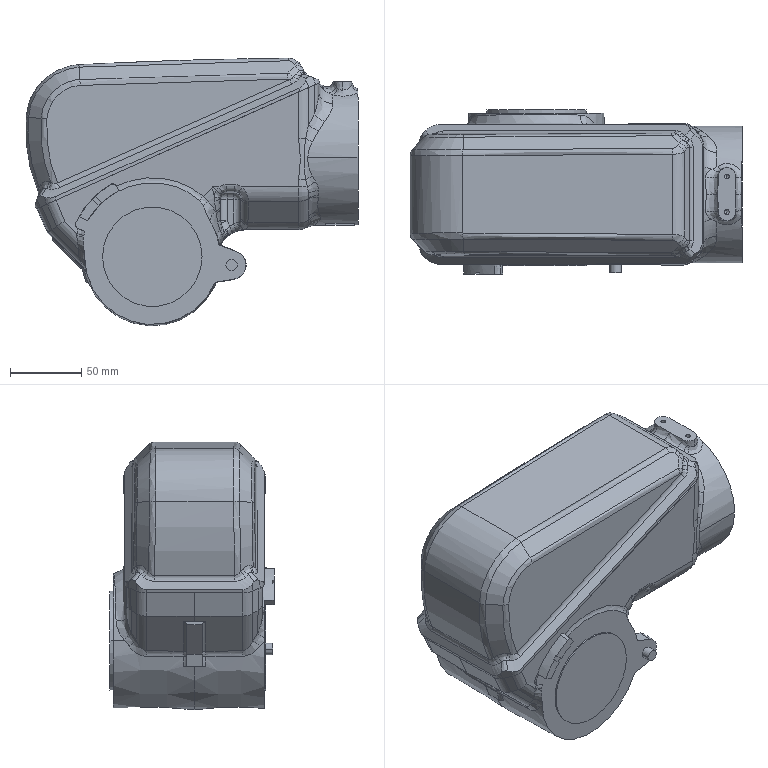Part | STEP file | ASND-0110-IRB120_3-58_IRC5_Link3_rev0-1 | 2 solids | 457 faces | box 233.871 x 115.5 x 188.155 mm | volume 2907846 mm3 | spline 196 | cylinder 106 | plane 98 | cone 36 | torus 10 | sphere 6 | other 5 | commonest cylinder face diameters 10 x24 20 x19 16 x10 17 x8 30 x6 40 x6